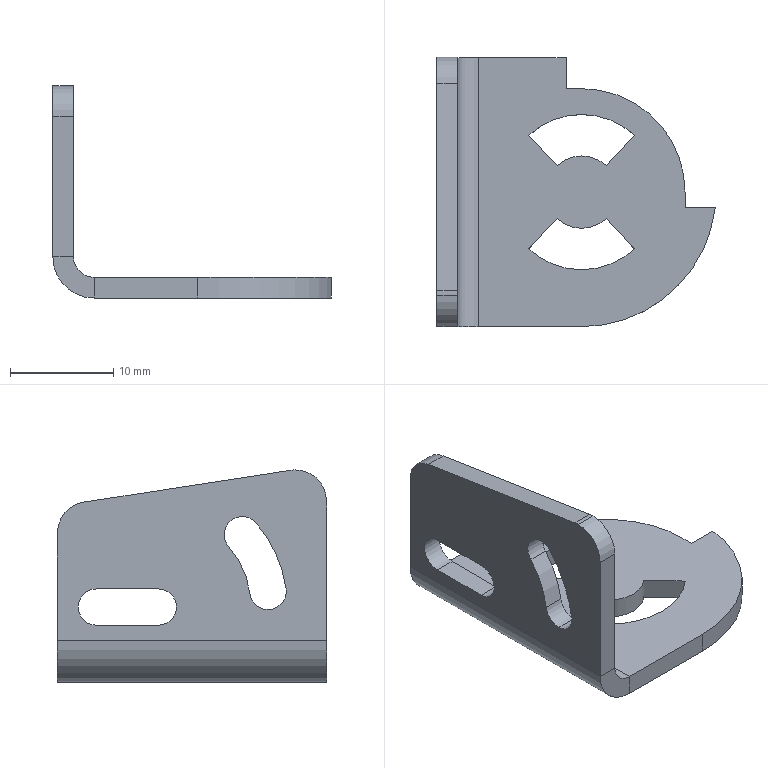Part | SolidWorks | features ICE 4, EdgeFlange 1, Fillet 1, FlatPattern 1, SMBaseFlange 1, SheetMetal 1 | 1 solid | 39 faces | box 26.913 x 26 x 20.503 mm | volume 1687 mm3 | plane 21 | cylinder 18 | commonest cylinder face diameters 3.5 x5 6 x3 7 x2 15 x2 4 x1 8 x1
STEP:
#1=CARTESIAN_POINT('',(-5.,-10.,18.503));
#2=VERTEX_POINT('',#1);
#3=CARTESIAN_POINT('',(-5.,-13.,15.503));
#4=VERTEX_POINT('',#3);
#5=CARTESIAN_POINT('',(-5.,-10.,15.503));
#6=DIRECTION('',(1.,0.,0.));
#7=DIRECTION('',(0.,0.,1.));
#8=AXIS2_PLACEMENT_3D('',#5,#6,#7);
#9=CIRCLE('',#8,3.);
#10=EDGE_CURVE('',#2,#4,#9,.T.);
#11=ORIENTED_EDGE('',*,*,#10,.F.);
#12=CARTESIAN_POINT('',(-7.,-10.,18.503));
#13=VERTEX_POINT('',#12);
#14=CARTESIAN_POINT('',(-7.,-10.,18.503));
#15=DIRECTION('',(-1.,0.,0.));
#16=VECTOR('',#15,1000.);
#17=LINE('',#14,#16);
#18=EDGE_CURVE('',#2,#13,#17,.T.);
#19=ORIENTED_EDGE('',*,*,#18,.T.);
#20=CARTESIAN_POINT('',(-7.,-13.,15.503));
#21=VERTEX_POINT('',#20);
#22=CARTESIAN_POINT('',(-7.,-10.,15.503));
#23=DIRECTION('',(-1.,0.,0.));
#24=DIRECTION('',(0.,0.,1.));
#25=AXIS2_PLACEMENT_3D('',#22,#23,#24);
#26=CIRCLE('',#25,3.);
#27=EDGE_CURVE('',#21,#13,#26,.T.);
#28=ORIENTED_EDGE('',*,*,#27,.F.);
#29=CARTESIAN_POINT('',(-7.,-13.,15.503));
#30=DIRECTION('',(-1.,0.,0.));
#31=VECTOR('',#30,1000.);
#32=LINE('',#29,#31);
#33=EDGE_CURVE('',#4,#21,#32,.T.);
#34=ORIENTED_EDGE('',*,*,#33,.F.);
#35=EDGE_LOOP('',(#11,#19,#28,#34));
#36=FACE_OUTER_BOUND('',#35,.T.);
#37=CARTESIAN_POINT('',(-7.,-10.,15.503));
#38=DIRECTION('',(-1.,0.,0.));
#39=DIRECTION('',(0.,0.,1.));
#40=AXIS2_PLACEMENT_3D('',#37,#38,#39);
#41=CYLINDRICAL_SURFACE('',#40,3.);
#42=ADVANCED_FACE('',(#36),#41,.T.);
#43=CARTESIAN_POINT('',(-7.,-7.354,5.));
#44=VERTEX_POINT('',#43);
#45=CARTESIAN_POINT('',(-7.,-5.621,6.505));
#46=VERTEX_POINT('',#45);
#47=CARTESIAN_POINT('',(-7.,-7.354,6.75));
#48=DIRECTION('',(1.,0.,0.));
#49=DIRECTION('',(0.,0.,-1.));
#50=AXIS2_PLACEMENT_3D('',#47,#48,#49);
#51=CIRCLE('',#50,1.75);
#52=EDGE_CURVE('',#44,#46,#51,.T.);
#53=ORIENTED_EDGE('',*,*,#52,.F.);
#54=CARTESIAN_POINT('',(-5.,-7.354,5.));
#55=VERTEX_POINT('',#54);
#56=CARTESIAN_POINT('',(-7.,-7.354,5.));
#57=DIRECTION('',(1.,0.,0.));
#58=VECTOR('',#57,1000.);
#59=LINE('',#56,#58);
#60=EDGE_CURVE('',#44,#55,#59,.T.);
#61=ORIENTED_EDGE('',*,*,#60,.T.);
#62=CARTESIAN_POINT('',(-5.,-5.621,6.505));
#63=VERTEX_POINT('',#62);
#64=CARTESIAN_POINT('',(-5.,-7.354,6.75));
#65=DIRECTION('',(1.,0.,0.));
#66=DIRECTION('',(0.,0.,-1.));
#67=AXIS2_PLACEMENT_3D('',#64,#65,#66);
#68=CIRCLE('',#67,1.75);
#69=EDGE_CURVE('',#55,#63,#68,.T.);
#70=ORIENTED_EDGE('',*,*,#69,.T.);
#71=CARTESIAN_POINT('',(-7.,-5.621,6.505));
#72=DIRECTION('',(1.,0.,0.));
#73=VECTOR('',#72,1000.);
#74=LINE('',#71,#73);
#75=EDGE_CURVE('',#46,#63,#74,.T.);
#76=ORIENTED_EDGE('',*,*,#75,.F.);
#77=EDGE_LOOP('',(#53,#61,#70,#76));
#78=FACE_OUTER_BOUND('',#77,.T.);
#79=CARTESIAN_POINT('',(-7.,-7.354,6.75));
#80=DIRECTION('',(1.,0.,0.));
#81=DIRECTION('',(0.,0.,-1.));
#82=AXIS2_PLACEMENT_3D('',#79,#80,#81);
#83=CYLINDRICAL_SURFACE('',#82,1.75);
#84=ADVANCED_FACE('',(#78),#83,.F.);
#85=CARTESIAN_POINT('',(-3.,-13.,0.));
#86=VERTEX_POINT('',#85);
#87=CARTESIAN_POINT('',(7.,-13.,0.));
#88=VERTEX_POINT('',#87);
#89=CARTESIAN_POINT('',(-7.,-13.,0.));
#90=DIRECTION('',(1.,0.,0.));
#91=VECTOR('',#90,1000.);
#92=LINE('',#89,#91);
#93=EDGE_CURVE('',#86,#88,#92,.T.);
#94=ORIENTED_EDGE('',*,*,#93,.F.);
#95=CARTESIAN_POINT('',(-3.,-13.,-2.));
#96=VERTEX_POINT('',#95);
#97=CARTESIAN_POINT('',(-3.,-13.,0.));
#98=DIRECTION('',(0.,0.,-1.));
#99=VECTOR('',#98,1000.);
#100=LINE('',#97,#99);
#101=EDGE_CURVE('',#86,#96,#100,.T.);
#102=ORIENTED_EDGE('',*,*,#101,.T.);
#103=CARTESIAN_POINT('',(7.,-13.,-2.));
#104=VERTEX_POINT('',#103);
#105=CARTESIAN_POINT('',(-7.,-13.,-2.));
#106=DIRECTION('',(1.,0.,0.));
#107=VECTOR('',#106,1000.);
#108=LINE('',#105,#107);
#109=EDGE_CURVE('',#96,#104,#108,.T.);
#110=ORIENTED_EDGE('',*,*,#109,.T.);
#111=CARTESIAN_POINT('',(7.,-13.,-2.));
#112=DIRECTION('',(0.,0.,1.));
#113=VECTOR('',#112,1000.);
#114=LINE('',#111,#113);
#115=EDGE_CURVE('',#104,#88,#114,.T.);
#116=ORIENTED_EDGE('',*,*,#115,.T.);
#117=EDGE_LOOP('',(#94,#102,#110,#116));
#118=FACE_OUTER_BOUND('',#117,.T.);
#119=CARTESIAN_POINT('',(-7.,-13.,-2.));
#120=DIRECTION('',(0.,-1.,0.));
#121=DIRECTION('',(0.,0.,-1.));
#122=AXIS2_PLACEMENT_3D('',#119,#120,#121);
#123=PLANE('',#122);
#124=ADVANCED_FACE('',(#118),#123,.T.);
#125=CARTESIAN_POINT('',(1.901,-5.5,-2.));
#126=VERTEX_POINT('',#125);
#127=CARTESIAN_POINT('',(12.099,-5.5,-2.));
#128=VERTEX_POINT('',#127);
#129=CARTESIAN_POINT('',(7.,0.,-2.));
#130=DIRECTION('',(0.,0.,1.));
#131=DIRECTION('',(-1.,0.,0.));
#132=AXIS2_PLACEMENT_3D('',#129,#130,#131);
#133=CIRCLE('',#132,7.5);
#134=EDGE_CURVE('',#126,#128,#133,.T.);
#135=ORIENTED_EDGE('',*,*,#134,.T.);
#136=CARTESIAN_POINT('',(9.38,-2.567,-2.));
#137=VERTEX_POINT('',#136);
#138=CARTESIAN_POINT('',(12.099,-5.5,-2.));
#139=DIRECTION('',(-0.6799,0.7333,0.));
#140=VECTOR('',#139,1000.);
#141=LINE('',#138,#140);
#142=EDGE_CURVE('',#128,#137,#141,.T.);
#143=ORIENTED_EDGE('',*,*,#142,.T.);
#144=CARTESIAN_POINT('',(4.62,-2.567,-2.));
#145=VERTEX_POINT('',#144);
#146=CARTESIAN_POINT('',(7.,0.,-2.));
#147=DIRECTION('',(0.,0.,-1.));
#148=DIRECTION('',(-1.,0.,0.));
#149=AXIS2_PLACEMENT_3D('',#146,#147,#148);
#150=CIRCLE('',#149,3.5);
#151=EDGE_CURVE('',#137,#145,#150,.T.);
#152=ORIENTED_EDGE('',*,*,#151,.T.);
#153=CARTESIAN_POINT('',(4.62,-2.567,-2.));
#154=DIRECTION('',(-0.6799,-0.7333,0.));
#155=VECTOR('',#154,1000.);
#156=LINE('',#153,#155);
#157=EDGE_CURVE('',#145,#126,#156,.T.);
#158=ORIENTED_EDGE('',*,*,#157,.T.);
#159=EDGE_LOOP('',(#135,#143,#152,#158));
#160=FACE_BOUND('',#159,.T.);
#161=CARTESIAN_POINT('',(4.62,2.567,-2.));
#162=VERTEX_POINT('',#161);
#163=CARTESIAN_POINT('',(9.38,2.567,-2.));
#164=VERTEX_POINT('',#163);
#165=CARTESIAN_POINT('',(7.,0.,-2.));
#166=DIRECTION('',(0.,0.,-1.));
#167=DIRECTION('',(1.,0.,0.));
#168=AXIS2_PLACEMENT_3D('',#165,#166,#167);
#169=CIRCLE('',#168,3.5);
#170=EDGE_CURVE('',#162,#164,#169,.T.);
#171=ORIENTED_EDGE('',*,*,#170,.T.);
#172=CARTESIAN_POINT('',(12.099,5.5,-2.));
#173=VERTEX_POINT('',#172);
#174=CARTESIAN_POINT('',(12.099,5.5,-2.));
#175=DIRECTION('',(0.6799,0.7333,0.));
#176=VECTOR('',#175,1000.);
#177=LINE('',#174,#176);
#178=EDGE_CURVE('',#164,#173,#177,.T.);
#179=ORIENTED_EDGE('',*,*,#178,.T.);
#180=CARTESIAN_POINT('',(1.901,5.5,-2.));
#181=VERTEX_POINT('',#180);
#182=CARTESIAN_POINT('',(7.,0.,-2.));
#183=DIRECTION('',(0.,0.,1.));
#184=DIRECTION('',(1.,0.,0.));
#185=AXIS2_PLACEMENT_3D('',#182,#183,#184);
#186=CIRCLE('',#185,7.5);
#187=EDGE_CURVE('',#173,#181,#186,.T.);
#188=ORIENTED_EDGE('',*,*,#187,.T.);
#189=CARTESIAN_POINT('',(4.62,2.567,-2.));
#190=DIRECTION('',(0.6799,-0.7333,0.));
#191=VECTOR('',#190,1000.);
#192=LINE('',#189,#191);
#193=EDGE_CURVE('',#181,#162,#192,.T.);
#194=ORIENTED_EDGE('',*,*,#193,.T.);
#195=EDGE_LOOP('',(#171,#179,#188,#194));
#196=FACE_BOUND('',#195,.T.);
#197=CARTESIAN_POINT('',(17.,-1.5,-2.));
#198=VERTEX_POINT('',#197);
#199=CARTESIAN_POINT('',(19.913,-1.5,-2.));
#200=VERTEX_POINT('',#199);
#201=CARTESIAN_POINT('',(17.,-1.5,-2.));
#202=DIRECTION('',(1.,0.,0.));
#203=VECTOR('',#202,1000.);
#204=LINE('',#201,#203);
#205=EDGE_CURVE('',#198,#200,#204,.T.);
#206=ORIENTED_EDGE('',*,*,#205,.T.);
#207=CARTESIAN_POINT('',(7.,0.,-2.));
#208=DIRECTION('',(0.,0.,1.));
#209=DIRECTION('',(-1.,0.,0.));
#210=AXIS2_PLACEMENT_3D('',#207,#208,#209);
#211=CIRCLE('',#210,13.);
#212=EDGE_CURVE('',#104,#200,#211,.T.);
#213=ORIENTED_EDGE('',*,*,#212,.F.);
#214=ORIENTED_EDGE('',*,*,#109,.F.);
#215=CARTESIAN_POINT('',(-3.,13.,-2.));
#216=VERTEX_POINT('',#215);
#217=CARTESIAN_POINT('',(-3.,-13.,-2.));
#218=DIRECTION('',(0.,1.,0.));
#219=VECTOR('',#218,1000.);
#220=LINE('',#217,#219);
#221=EDGE_CURVE('',#96,#216,#220,.T.);
#222=ORIENTED_EDGE('',*,*,#221,.T.);
#223=CARTESIAN_POINT('',(5.5,13.,-2.));
#224=VERTEX_POINT('',#223);
#225=CARTESIAN_POINT('',(-7.,13.,-2.));
#226=DIRECTION('',(-1.,0.,0.));
#227=VECTOR('',#226,1000.);
#228=LINE('',#225,#227);
#229=EDGE_CURVE('',#224,#216,#228,.T.);
#230=ORIENTED_EDGE('',*,*,#229,.F.);
#231=CARTESIAN_POINT('',(5.5,10.,-2.));
#232=VERTEX_POINT('',#231);
#233=CARTESIAN_POINT('',(5.5,13.,-2.));
#234=DIRECTION('',(0.,-1.,0.));
#235=VECTOR('',#234,1000.);
#236=LINE('',#233,#235);
#237=EDGE_CURVE('',#224,#232,#236,.T.);
#238=ORIENTED_EDGE('',*,*,#237,.T.);
#239=CARTESIAN_POINT('',(7.,10.,-2.));
#240=VERTEX_POINT('',#239);
#241=CARTESIAN_POINT('',(5.5,10.,-2.));
#242=DIRECTION('',(1.,0.,0.));
#243=VECTOR('',#242,1000.);
#244=LINE('',#241,#243);
#245=EDGE_CURVE('',#232,#240,#244,.T.);
#246=ORIENTED_EDGE('',*,*,#245,.T.);
#247=CARTESIAN_POINT('',(17.,0.,-2.));
#248=VERTEX_POINT('',#247);
#249=CARTESIAN_POINT('',(7.,0.,-2.));
#250=DIRECTION('',(0.,0.,-1.));
#251=DIRECTION('',(1.,0.,0.));
#252=AXIS2_PLACEMENT_3D('',#249,#250,#251);
#253=CIRCLE('',#252,10.);
#254=EDGE_CURVE('',#240,#248,#253,.T.);
#255=ORIENTED_EDGE('',*,*,#254,.T.);
#256=CARTESIAN_POINT('',(17.,0.,-2.));
#257=DIRECTION('',(0.,-1.,0.));
#258=VECTOR('',#257,1000.);
#259=LINE('',#256,#258);
#260=EDGE_CURVE('',#248,#198,#259,.T.);
#261=ORIENTED_EDGE('',*,*,#260,.T.);
#262=EDGE_LOOP('',(#206,#213,#214,#222,#230,#238,#246,#255,#261));
#263=FACE_OUTER_BOUND('',#262,.T.);
#264=CARTESIAN_POINT('',(7.,0.,-2.));
#265=DIRECTION('',(0.,0.,-1.));
#266=DIRECTION('',(-1.,0.,0.));
#267=AXIS2_PLACEMENT_3D('',#264,#265,#266);
#268=PLANE('',#267);
#269=ADVANCED_FACE('',(#160,#196,#263),#268,.T.);
#270=CARTESIAN_POINT('',(12.099,-5.5,0.));
#271=VERTEX_POINT('',#270);
#272=CARTESIAN_POINT('',(9.38,-2.567,0.));
#273=VERTEX_POINT('',#272);
#274=CARTESIAN_POINT('',(12.099,-5.5,0.));
#275=DIRECTION('',(-0.6799,0.7333,0.));
#276=VECTOR('',#275,1000.);
#277=LINE('',#274,#276);
#278=EDGE_CURVE('',#271,#273,#277,.T.);
#279=ORIENTED_EDGE('',*,*,#278,.F.);
#280=CARTESIAN_POINT('',(1.901,-5.5,0.));
#281=VERTEX_POINT('',#280);
#282=CARTESIAN_POINT('',(7.,0.,0.));
#283=DIRECTION('',(0.,0.,1.));
#284=DIRECTION('',(-1.,0.,0.));
#285=AXIS2_PLACEMENT_3D('',#282,#283,#284);
#286=CIRCLE('',#285,7.5);
#287=EDGE_CURVE('',#281,#271,#286,.T.);
#288=ORIENTED_EDGE('',*,*,#287,.F.);
#289=CARTESIAN_POINT('',(4.62,-2.567,0.));
#290=VERTEX_POINT('',#289);
#291=CARTESIAN_POINT('',(4.62,-2.567,0.));
#292=DIRECTION('',(-0.6799,-0.7333,0.));
#293=VECTOR('',#292,1000.);
#294=LINE('',#291,#293);
#295=EDGE_CURVE('',#290,#281,#294,.T.);
#296=ORIENTED_EDGE('',*,*,#295,.F.);
#297=CARTESIAN_POINT('',(7.,0.,0.));
#298=DIRECTION('',(0.,0.,-1.));
#299=DIRECTION('',(-1.,0.,0.));
#300=AXIS2_PLACEMENT_3D('',#297,#298,#299);
#301=CIRCLE('',#300,3.5);
#302=EDGE_CURVE('',#273,#290,#301,.T.);
#303=ORIENTED_EDGE('',*,*,#302,.F.);
#304=EDGE_LOOP('',(#279,#288,#296,#303));
#305=FACE_BOUND('',#304,.T.);
#306=CARTESIAN_POINT('',(9.38,2.567,0.));
#307=VERTEX_POINT('',#306);
#308=CARTESIAN_POINT('',(12.099,5.5,0.));
#309=VERTEX_POINT('',#308);
#310=CARTESIAN_POINT('',(12.099,5.5,0.));
#311=DIRECTION('',(0.6799,0.7333,0.));
#312=VECTOR('',#311,1000.);
#313=LINE('',#310,#312);
#314=EDGE_CURVE('',#307,#309,#313,.T.);
#315=ORIENTED_EDGE('',*,*,#314,.F.);
#316=CARTESIAN_POINT('',(4.62,2.567,0.));
#317=VERTEX_POINT('',#316);
#318=CARTESIAN_POINT('',(7.,0.,0.));
#319=DIRECTION('',(0.,0.,-1.));
#320=DIRECTION('',(1.,0.,0.));
#321=AXIS2_PLACEMENT_3D('',#318,#319,#320);
#322=CIRCLE('',#321,3.5);
#323=EDGE_CURVE('',#317,#307,#322,.T.);
#324=ORIENTED_EDGE('',*,*,#323,.F.);
#325=CARTESIAN_POINT('',(1.901,5.5,0.));
#326=VERTEX_POINT('',#325);
#327=CARTESIAN_POINT('',(4.62,2.567,0.));
#328=DIRECTION('',(0.6799,-0.7333,0.));
#329=VECTOR('',#328,1000.);
#330=LINE('',#327,#329);
#331=EDGE_CURVE('',#326,#317,#330,.T.);
#332=ORIENTED_EDGE('',*,*,#331,.F.);
#333=CARTESIAN_POINT('',(7.,0.,0.));
#334=DIRECTION('',(0.,0.,1.));
#335=DIRECTION('',(1.,0.,0.));
#336=AXIS2_PLACEMENT_3D('',#333,#334,#335);
#337=CIRCLE('',#336,7.5);
#338=EDGE_CURVE('',#309,#326,#337,.T.);
#339=ORIENTED_EDGE('',*,*,#338,.F.);
#340=EDGE_LOOP('',(#315,#324,#332,#339));
#341=FACE_BOUND('',#340,.T.);
#342=CARTESIAN_POINT('',(19.913,-1.5,0.));
#343=VERTEX_POINT('',#342);
#344=CARTESIAN_POINT('',(7.,0.,0.));
#345=DIRECTION('',(0.,0.,1.));
#346=DIRECTION('',(-1.,0.,0.));
#347=AXIS2_PLACEMENT_3D('',#344,#345,#346);
#348=CIRCLE('',#347,13.);
#349=EDGE_CURVE('',#88,#343,#348,.T.);
#350=ORIENTED_EDGE('',*,*,#349,.T.);
#351=CARTESIAN_POINT('',(17.,-1.5,0.));
#352=VERTEX_POINT('',#351);
#353=CARTESIAN_POINT('',(17.,-1.5,0.));
#354=DIRECTION('',(1.,0.,0.));
#355=VECTOR('',#354,1000.);
#356=LINE('',#353,#355);
#357=EDGE_CURVE('',#352,#343,#356,.T.);
#358=ORIENTED_EDGE('',*,*,#357,.F.);
#359=CARTESIAN_POINT('',(17.,0.,0.));
#360=VERTEX_POINT('',#359);
#361=CARTESIAN_POINT('',(17.,0.,0.));
#362=DIRECTION('',(0.,-1.,0.));
#363=VECTOR('',#362,1000.);
#364=LINE('',#361,#363);
#365=EDGE_CURVE('',#360,#352,#364,.T.);
#366=ORIENTED_EDGE('',*,*,#365,.F.);
#367=CARTESIAN_POINT('',(7.,10.,0.));
#368=VERTEX_POINT('',#367);
#369=CARTESIAN_POINT('',(7.,0.,0.));
#370=DIRECTION('',(0.,0.,-1.));
#371=DIRECTION('',(1.,0.,0.));
#372=AXIS2_PLACEMENT_3D('',#369,#370,#371);
#373=CIRCLE('',#372,10.);
#374=EDGE_CURVE('',#368,#360,#373,.T.);
#375=ORIENTED_EDGE('',*,*,#374,.F.);
#376=CARTESIAN_POINT('',(5.5,10.,0.));
#377=VERTEX_POINT('',#376);
#378=CARTESIAN_POINT('',(5.5,10.,0.));
#379=DIRECTION('',(1.,0.,0.));
#380=VECTOR('',#379,1000.);
#381=LINE('',#378,#380);
#382=EDGE_CURVE('',#377,#368,#381,.T.);
#383=ORIENTED_EDGE('',*,*,#382,.F.);
#384=CARTESIAN_POINT('',(5.5,13.,0.));
#385=VERTEX_POINT('',#384);
#386=CARTESIAN_POINT('',(5.5,13.,0.));
#387=DIRECTION('',(0.,-1.,0.));
#388=VECTOR('',#387,1000.);
#389=LINE('',#386,#388);
#390=EDGE_CURVE('',#385,#377,#389,.T.);
#391=ORIENTED_EDGE('',*,*,#390,.F.);
#392=CARTESIAN_POINT('',(-3.,13.,0.));
#393=VERTEX_POINT('',#392);
#394=CARTESIAN_POINT('',(-7.,13.,0.));
#395=DIRECTION('',(-1.,0.,0.));
#396=VECTOR('',#395,1000.);
#397=LINE('',#394,#396);
#398=EDGE_CURVE('',#385,#393,#397,.T.);
#399=ORIENTED_EDGE('',*,*,#398,.T.);
#400=CARTESIAN_POINT('',(-3.,-13.,0.));
#401=DIRECTION('',(0.,1.,0.));
#402=VECTOR('',#401,1000.);
#403=LINE('',#400,#402);
#404=EDGE_CURVE('',#86,#393,#403,.T.);
#405=ORIENTED_EDGE('',*,*,#404,.F.);
#406=ORIENTED_EDGE('',*,*,#93,.T.);
#407=EDGE_LOOP('',(#350,#358,#366,#375,#383,#391,#399,#405,#406));
#408=FACE_OUTER_BOUND('',#407,.T.);
#409=CARTESIAN_POINT('',(7.,0.,0.));
#410=DIRECTION('',(0.,0.,-1.));
#411=DIRECTION('',(-1.,0.,0.));
#412=AXIS2_PLACEMENT_3D('',#409,#410,#411);
#413=PLANE('',#412);
#414=ADVANCED_FACE('',(#305,#341,#408),#413,.F.);
#415=CARTESIAN_POINT('',(19.913,-1.5,-2.));
#416=DIRECTION('',(0.,0.,1.));
#417=VECTOR('',#416,1000.);
#418=LINE('',#415,#417);
#419=EDGE_CURVE('',#200,#343,#418,.T.);
#420=ORIENTED_EDGE('',*,*,#419,.T.);
#421=ORIENTED_EDGE('',*,*,#349,.F.);
#422=ORIENTED_EDGE('',*,*,#115,.F.);
#423=ORIENTED_EDGE('',*,*,#212,.T.);
#424=EDGE_LOOP('',(#420,#421,#422,#423));
#425=FACE_OUTER_BOUND('',#424,.T.);
#426=CARTESIAN_POINT('',(7.,0.,-2.));
#427=DIRECTION('',(0.,0.,1.));
#428=DIRECTION('',(1.,0.,0.));
#429=AXIS2_PLACEMENT_3D('',#426,#427,#428);
#430=CYLINDRICAL_SURFACE('',#429,13.);
#431=ADVANCED_FACE('',(#425),#430,.T.);
#432=CARTESIAN_POINT('',(5.5,13.,-2.));
#433=DIRECTION('',(0.,0.,1.));
#434=VECTOR('',#433,1000.);
#435=LINE('',#432,#434);
#436=EDGE_CURVE('',#224,#385,#435,.T.);
#437=ORIENTED_EDGE('',*,*,#436,.F.);
#438=ORIENTED_EDGE('',*,*,#229,.T.);
#439=CARTESIAN_POINT('',(-3.,13.,0.));
#440=DIRECTION('',(0.,0.,-1.));
#441=VECTOR('',#440,1000.);
#442=LINE('',#439,#441);
#443=EDGE_CURVE('',#393,#216,#442,.T.);
#444=ORIENTED_EDGE('',*,*,#443,.F.);
#445=ORIENTED_EDGE('',*,*,#398,.F.);
#446=EDGE_LOOP('',(#437,#438,#444,#445));
#447=FACE_OUTER_BOUND('',#446,.T.);
#448=CARTESIAN_POINT('',(-7.,13.,-2.));
#449=DIRECTION('',(0.,1.,0.));
#450=DIRECTION('',(0.,0.,1.));
#451=AXIS2_PLACEMENT_3D('',#448,#449,#450);
#452=PLANE('',#451);
#453=ADVANCED_FACE('',(#447),#452,.T.);
#454=CARTESIAN_POINT('',(-5.,13.,2.));
#455=VERTEX_POINT('',#454);
#456=CARTESIAN_POINT('',(-7.,13.,2.));
#457=VERTEX_POINT('',#456);
#458=CARTESIAN_POINT('',(-7.,13.,2.));
#459=DIRECTION('',(-1.,0.,0.));
#460=VECTOR('',#459,1000.);
#461=LINE('',#458,#460);
#462=EDGE_CURVE('',#455,#457,#461,.T.);
#463=ORIENTED_EDGE('',*,*,#462,.F.);
#464=CARTESIAN_POINT('',(-3.,13.,2.));
#465=DIRECTION('',(0.,1.,0.));
#466=DIRECTION('',(0.,0.,-1.));
#467=AXIS2_PLACEMENT_3D('',#464,#465,#466);
#468=CIRCLE('',#467,2.);
#469=EDGE_CURVE('',#393,#455,#468,.T.);
#470=ORIENTED_EDGE('',*,*,#469,.F.);
#471=ORIENTED_EDGE('',*,*,#443,.T.);
#472=CARTESIAN_POINT('',(-3.,13.,2.));
#473=DIRECTION('',(0.,1.,0.));
#474=DIRECTION('',(0.,0.,-1.));
#475=AXIS2_PLACEMENT_3D('',#472,#473,#474);
#476=CIRCLE('',#475,4.);
#477=EDGE_CURVE('',#216,#457,#476,.T.);
#478=ORIENTED_EDGE('',*,*,#477,.T.);
#479=EDGE_LOOP('',(#463,#470,#471,#478));
#480=FACE_OUTER_BOUND('',#479,.T.);
#481=CARTESIAN_POINT('',(-3.,13.,2.));
#482=DIRECTION('',(0.,1.,0.));
#483=DIRECTION('',(0.,0.,1.));
#484=AXIS2_PLACEMENT_3D('',#481,#482,#483);
#485=PLANE('',#484);
#486=ADVANCED_FACE('',(#480),#485,.T.);
#487=CARTESIAN_POINT('',(-5.,-13.,2.));
#488=VERTEX_POINT('',#487);
#489=CARTESIAN_POINT('',(-3.,-13.,2.));
#490=DIRECTION('',(0.,-1.,0.));
#491=DIRECTION('',(0.,0.,-1.));
#492=AXIS2_PLACEMENT_3D('',#489,#490,#491);
#493=CIRCLE('',#492,2.);
#494=EDGE_CURVE('',#488,#86,#493,.T.);
#495=ORIENTED_EDGE('',*,*,#494,.F.);
#496=CARTESIAN_POINT('',(-7.,-13.,2.));
#497=VERTEX_POINT('',#496);
#498=CARTESIAN_POINT('',(-5.,-13.,2.));
#499=DIRECTION('',(-1.,0.,0.));
#500=VECTOR('',#499,1000.);
#501=LINE('',#498,#500);
#502=EDGE_CURVE('',#488,#497,#501,.T.);
#503=ORIENTED_EDGE('',*,*,#502,.T.);
#504=CARTESIAN_POINT('',(-3.,-13.,2.));
#505=DIRECTION('',(0.,-1.,0.));
#506=DIRECTION('',(0.,0.,-1.));
#507=AXIS2_PLACEMENT_3D('',#504,#505,#506);
#508=CIRCLE('',#507,4.);
#509=EDGE_CURVE('',#497,#96,#508,.T.);
#510=ORIENTED_EDGE('',*,*,#509,.T.);
#511=ORIENTED_EDGE('',*,*,#101,.F.);
#512=EDGE_LOOP('',(#495,#503,#510,#511));
#513=FACE_OUTER_BOUND('',#512,.T.);
#514=CARTESIAN_POINT('',(-3.,-13.,2.));
#515=DIRECTION('',(0.,1.,0.));
#516=DIRECTION('',(0.,0.,1.));
#517=AXIS2_PLACEMENT_3D('',#514,#515,#516);
#518=PLANE('',#517);
#519=ADVANCED_FACE('',(#513),#518,.F.);
#520=ORIENTED_EDGE('',*,*,#221,.F.);
#521=ORIENTED_EDGE('',*,*,#509,.F.);
#522=CARTESIAN_POINT('',(-7.,0.,2.));
#523=DIRECTION('',(0.,-1.,0.));
#524=VECTOR('',#523,1000.);
#525=LINE('',#522,#524);
#526=EDGE_CURVE('',#457,#497,#525,.T.);
#527=ORIENTED_EDGE('',*,*,#526,.F.);
#528=ORIENTED_EDGE('',*,*,#477,.F.);
#529=EDGE_LOOP('',(#520,#521,#527,#528));
#530=FACE_OUTER_BOUND('',#529,.T.);
#531=CARTESIAN_POINT('',(-3.,-13.,2.));
#532=DIRECTION('',(0.,-1.,0.));
#533=DIRECTION('',(-1.,0.,0.));
#534=AXIS2_PLACEMENT_3D('',#531,#532,#533);
#535=CYLINDRICAL_SURFACE('',#534,4.);
#536=ADVANCED_FACE('',(#530),#535,.T.);
#537=ORIENTED_EDGE('',*,*,#404,.T.);
#538=ORIENTED_EDGE('',*,*,#469,.T.);
#539=CARTESIAN_POINT('',(-5.,13.,2.));
#540=DIRECTION('',(0.,-1.,0.));
#541=VECTOR('',#540,1000.);
#542=LINE('',#539,#541);
#543=EDGE_CURVE('',#455,#488,#542,.T.);
#544=ORIENTED_EDGE('',*,*,#543,.T.);
#545=ORIENTED_EDGE('',*,*,#494,.T.);
#546=EDGE_LOOP('',(#537,#538,#544,#545));
#547=FACE_OUTER_BOUND('',#546,.T.);
#548=CARTESIAN_POINT('',(-3.,-13.,2.));
#549=DIRECTION('',(0.,-1.,0.));
#550=DIRECTION('',(-1.,0.,0.));
#551=AXIS2_PLACEMENT_3D('',#548,#549,#550);
#552=CYLINDRICAL_SURFACE('',#551,2.);
#553=ADVANCED_FACE('',(#547),#552,.F.);
#554=CARTESIAN_POINT('',(-5.,-13.,0.));
#555=DIRECTION('',(0.,0.,-1.));
#556=VECTOR('',#555,1000.);
#557=LINE('',#554,#556);
#558=EDGE_CURVE('',#4,#488,#557,.T.);
#559=ORIENTED_EDGE('',*,*,#558,.F.);
#560=ORIENTED_EDGE('',*,*,#33,.T.);
#561=CARTESIAN_POINT('',(-7.,-13.,0.));
#562=DIRECTION('',(0.,0.,-1.));
#563=VECTOR('',#562,1000.);
#564=LINE('',#561,#563);
#565=EDGE_CURVE('',#21,#497,#564,.T.);
#566=ORIENTED_EDGE('',*,*,#565,.T.);
#567=ORIENTED_EDGE('',*,*,#502,.F.);
#568=EDGE_LOOP('',(#559,#560,#566,#567));
#569=FACE_OUTER_BOUND('',#568,.T.);
#570=CARTESIAN_POINT('',(-7.,-13.,0.));
#571=DIRECTION('',(0.,-1.,0.));
#572=DIRECTION('',(0.,0.,-1.));
#573=AXIS2_PLACEMENT_3D('',#570,#571,#572);
#574=PLANE('',#573);
#575=ADVANCED_FACE('',(#569),#574,.T.);
#576=CARTESIAN_POINT('',(-7.,13.,12.426));
#577=VERTEX_POINT('',#576);
#578=CARTESIAN_POINT('',(-7.,13.,19.));
#579=DIRECTION('',(0.,0.,1.));
#580=VECTOR('',#579,1000.);
#581=LINE('',#578,#580);
#582=EDGE_CURVE('',#457,#577,#581,.T.);
#583=ORIENTED_EDGE('',*,*,#582,.T.);
#584=CARTESIAN_POINT('',(-5.,13.,12.426));
#585=VERTEX_POINT('',#584);
#586=CARTESIAN_POINT('',(-5.,13.,12.426));
#587=DIRECTION('',(1.,0.,0.));
#588=VECTOR('',#587,1000.);
#589=LINE('',#586,#588);
#590=EDGE_CURVE('',#577,#585,#589,.T.);
#591=ORIENTED_EDGE('',*,*,#590,.T.);
#592=CARTESIAN_POINT('',(-5.,13.,0.));
#593=DIRECTION('',(0.,0.,1.));
#594=VECTOR('',#593,1000.);
#595=LINE('',#592,#594);
#596=EDGE_CURVE('',#455,#585,#595,.T.);
#597=ORIENTED_EDGE('',*,*,#596,.F.);
#598=ORIENTED_EDGE('',*,*,#462,.T.);
#599=EDGE_LOOP('',(#583,#591,#597,#598));
#600=FACE_OUTER_BOUND('',#599,.T.);
#601=CARTESIAN_POINT('',(-7.,13.,19.));
#602=DIRECTION('',(0.,1.,0.));
#603=DIRECTION('',(0.,0.,1.));
#604=AXIS2_PLACEMENT_3D('',#601,#602,#603);
#605=PLANE('',#604);
#606=ADVANCED_FACE('',(#600),#605,.T.);
#607=CARTESIAN_POINT('',(-7.,-9.544,18.468));
#608=VERTEX_POINT('',#607);
#609=CARTESIAN_POINT('',(-7.,10.456,15.391));
#610=VERTEX_POINT('',#609);
#611=CARTESIAN_POINT('',(-7.,-13.,19.));
#612=DIRECTION('',(0.,0.9884,-0.1521));
#613=VECTOR('',#612,1000.);
#614=LINE('',#611,#613);
#615=EDGE_CURVE('',#608,#610,#614,.T.);
#616=ORIENTED_EDGE('',*,*,#615,.T.);
#617=CARTESIAN_POINT('',(-7.,10.,12.426));
#618=DIRECTION('',(-1.,0.,0.));
#619=DIRECTION('',(0.,0.,1.));
#620=AXIS2_PLACEMENT_3D('',#617,#618,#619);
#621=CIRCLE('',#620,3.);
#622=EDGE_CURVE('',#610,#577,#621,.T.);
#623=ORIENTED_EDGE('',*,*,#622,.T.);
#624=ORIENTED_EDGE('',*,*,#582,.F.);
#625=ORIENTED_EDGE('',*,*,#526,.T.);
#626=ORIENTED_EDGE('',*,*,#565,.F.);
#627=ORIENTED_EDGE('',*,*,#27,.T.);
#628=CARTESIAN_POINT('',(-7.,-10.,15.503));
#629=DIRECTION('',(-1.,0.,0.));
#630=DIRECTION('',(0.,0.,1.));
#631=AXIS2_PLACEMENT_3D('',#628,#629,#630);
#632=CIRCLE('',#631,3.);
#633=EDGE_CURVE('',#13,#608,#632,.T.);
#634=ORIENTED_EDGE('',*,*,#633,.T.);
#635=EDGE_LOOP('',(#616,#623,#624,#625,#626,#627,#634));
#636=FACE_OUTER_BOUND('',#635,.T.);
#637=CARTESIAN_POINT('',(-7.,-3.53,11.106));
#638=VERTEX_POINT('',#637);
#639=CARTESIAN_POINT('',(-7.,-6.179,13.394));
#640=VERTEX_POINT('',#639);
#641=CARTESIAN_POINT('',(-7.,-4.855,12.25));
#642=DIRECTION('',(1.,0.,0.));
#643=DIRECTION('',(0.,0.,-1.));
#644=AXIS2_PLACEMENT_3D('',#641,#642,#643);
#645=CIRCLE('',#644,1.75);
#646=EDGE_CURVE('',#638,#640,#645,.T.);
#647=ORIENTED_EDGE('',*,*,#646,.T.);
#648=CARTESIAN_POINT('',(-7.,-9.086,6.995));
#649=VERTEX_POINT('',#648);
#650=CARTESIAN_POINT('',(-7.,3.25,5.25));
#651=DIRECTION('',(1.,0.,0.));
#652=DIRECTION('',(0.,0.,-1.));
#653=AXIS2_PLACEMENT_3D('',#650,#651,#652);
#654=CIRCLE('',#653,12.459);
#655=EDGE_CURVE('',#640,#649,#654,.T.);
#656=ORIENTED_EDGE('',*,*,#655,.T.);
#657=CARTESIAN_POINT('',(-7.,-7.354,6.75));
#658=DIRECTION('',(1.,0.,0.));
#659=DIRECTION('',(0.,0.,-1.));
#660=AXIS2_PLACEMENT_3D('',#657,#658,#659);
#661=CIRCLE('',#660,1.75);
#662=EDGE_CURVE('',#649,#44,#661,.T.);
#663=ORIENTED_EDGE('',*,*,#662,.T.);
#664=ORIENTED_EDGE('',*,*,#52,.T.);
#665=CARTESIAN_POINT('',(-7.,3.25,5.25));
#666=DIRECTION('',(-1.,0.,0.));
#667=DIRECTION('',(0.,0.,-1.));
#668=AXIS2_PLACEMENT_3D('',#665,#666,#667);
#669=CIRCLE('',#668,8.959);
#670=EDGE_CURVE('',#46,#638,#669,.T.);
#671=ORIENTED_EDGE('',*,*,#670,.T.);
#672=EDGE_LOOP('',(#647,#656,#663,#664,#671));
#673=FACE_BOUND('',#672,.T.);
#674=CARTESIAN_POINT('',(-7.,3.25,7.));
#675=VERTEX_POINT('',#674);
#676=CARTESIAN_POINT('',(-7.,3.25,3.5));
#677=VERTEX_POINT('',#676);
#678=CARTESIAN_POINT('',(-7.,3.25,5.25));
#679=DIRECTION('',(1.,0.,0.));
#680=DIRECTION('',(0.,0.,-1.));
#681=AXIS2_PLACEMENT_3D('',#678,#679,#680);
#682=CIRCLE('',#681,1.75);
#683=EDGE_CURVE('',#675,#677,#682,.T.);
#684=ORIENTED_EDGE('',*,*,#683,.T.);
#685=CARTESIAN_POINT('',(-7.,9.25,3.5));
#686=VERTEX_POINT('',#685);
#687=CARTESIAN_POINT('',(-7.,3.25,3.5));
#688=DIRECTION('',(0.,1.,0.));
#689=VECTOR('',#688,1000.);
#690=LINE('',#687,#689);
#691=EDGE_CURVE('',#677,#686,#690,.T.);
#692=ORIENTED_EDGE('',*,*,#691,.T.);
#693=CARTESIAN_POINT('',(-7.,9.25,7.));
#694=VERTEX_POINT('',#693);
#695=CARTESIAN_POINT('',(-7.,9.25,5.25));
#696=DIRECTION('',(1.,0.,0.));
#697=DIRECTION('',(0.,0.,-1.));
#698=AXIS2_PLACEMENT_3D('',#695,#696,#697);
#699=CIRCLE('',#698,1.75);
#700=EDGE_CURVE('',#686,#694,#699,.T.);
#701=ORIENTED_EDGE('',*,*,#700,.T.);
#702=CARTESIAN_POINT('',(-7.,3.25,7.));
#703=DIRECTION('',(0.,-1.,0.));
#704=VECTOR('',#703,1000.);
#705=LINE('',#702,#704);
#706=EDGE_CURVE('',#694,#675,#705,.T.);
#707=ORIENTED_EDGE('',*,*,#706,.T.);
#708=EDGE_LOOP('',(#684,#692,#701,#707));
#709=FACE_BOUND('',#708,.T.);
#710=CARTESIAN_POINT('',(-7.,0.,0.));
#711=DIRECTION('',(-1.,0.,0.));
#712=DIRECTION('',(0.,0.,1.));
#713=AXIS2_PLACEMENT_3D('',#710,#711,#712);
#714=PLANE('',#713);
#715=ADVANCED_FACE('',(#636,#673,#709),#714,.T.);
#716=CARTESIAN_POINT('',(-5.,-6.179,13.394));
#717=VERTEX_POINT('',#716);
#718=CARTESIAN_POINT('',(-5.,-9.086,6.995));
#719=VERTEX_POINT('',#718);
#720=CARTESIAN_POINT('',(-5.,3.25,5.25));
#721=DIRECTION('',(1.,0.,0.));
#722=DIRECTION('',(0.,0.,-1.));
#723=AXIS2_PLACEMENT_3D('',#720,#721,#722);
#724=CIRCLE('',#723,12.459);
#725=EDGE_CURVE('',#717,#719,#724,.T.);
#726=ORIENTED_EDGE('',*,*,#725,.F.);
#727=CARTESIAN_POINT('',(-5.,-3.53,11.106));
#728=VERTEX_POINT('',#727);
#729=CARTESIAN_POINT('',(-5.,-4.855,12.25));
#730=DIRECTION('',(1.,0.,0.));
#731=DIRECTION('',(0.,0.,-1.));
#732=AXIS2_PLACEMENT_3D('',#729,#730,#731);
#733=CIRCLE('',#732,1.75);
#734=EDGE_CURVE('',#728,#717,#733,.T.);
#735=ORIENTED_EDGE('',*,*,#734,.F.);
#736=CARTESIAN_POINT('',(-5.,3.25,5.25));
#737=DIRECTION('',(-1.,0.,0.));
#738=DIRECTION('',(0.,0.,-1.));
#739=AXIS2_PLACEMENT_3D('',#736,#737,#738);
#740=CIRCLE('',#739,8.959);
#741=EDGE_CURVE('',#63,#728,#740,.T.);
#742=ORIENTED_EDGE('',*,*,#741,.F.);
#743=ORIENTED_EDGE('',*,*,#69,.F.);
#744=CARTESIAN_POINT('',(-5.,-7.354,6.75));
#745=DIRECTION('',(1.,0.,0.));
#746=DIRECTION('',(0.,0.,-1.));
#747=AXIS2_PLACEMENT_3D('',#744,#745,#746);
#748=CIRCLE('',#747,1.75);
#749=EDGE_CURVE('',#719,#55,#748,.T.);
#750=ORIENTED_EDGE('',*,*,#749,.F.);
#751=EDGE_LOOP('',(#726,#735,#742,#743,#750));
#752=FACE_BOUND('',#751,.T.);
#753=CARTESIAN_POINT('',(-5.,3.25,3.5));
#754=VERTEX_POINT('',#753);
#755=CARTESIAN_POINT('',(-5.,9.25,3.5));
#756=VERTEX_POINT('',#755);
#757=CARTESIAN_POINT('',(-5.,3.25,3.5));
#758=DIRECTION('',(0.,1.,0.));
#759=VECTOR('',#758,1000.);
#760=LINE('',#757,#759);
#761=EDGE_CURVE('',#754,#756,#760,.T.);
#762=ORIENTED_EDGE('',*,*,#761,.F.);
#763=CARTESIAN_POINT('',(-5.,3.25,7.));
#764=VERTEX_POINT('',#763);
#765=CARTESIAN_POINT('',(-5.,3.25,5.25));
#766=DIRECTION('',(1.,0.,0.));
#767=DIRECTION('',(0.,0.,-1.));
#768=AXIS2_PLACEMENT_3D('',#765,#766,#767);
#769=CIRCLE('',#768,1.75);
#770=EDGE_CURVE('',#764,#754,#769,.T.);
#771=ORIENTED_EDGE('',*,*,#770,.F.);
#772=CARTESIAN_POINT('',(-5.,9.25,7.));
#773=VERTEX_POINT('',#772);
#774=CARTESIAN_POINT('',(-5.,3.25,7.));
#775=DIRECTION('',(0.,-1.,0.));
#776=VECTOR('',#775,1000.);
#777=LINE('',#774,#776);
#778=EDGE_CURVE('',#773,#764,#777,.T.);
#779=ORIENTED_EDGE('',*,*,#778,.F.);
#780=CARTESIAN_POINT('',(-5.,9.25,5.25));
#781=DIRECTION('',(1.,0.,0.));
#782=DIRECTION('',(0.,0.,-1.));
#783=AXIS2_PLACEMENT_3D('',#780,#781,#782);
#784=CIRCLE('',#783,1.75);
#785=EDGE_CURVE('',#756,#773,#784,.T.);
#786=ORIENTED_EDGE('',*,*,#785,.F.);
#787=EDGE_LOOP('',(#762,#771,#779,#786));
#788=FACE_BOUND('',#787,.T.);
#789=ORIENTED_EDGE('',*,*,#596,.T.);
#790=CARTESIAN_POINT('',(-5.,10.456,15.391));
#791=VERTEX_POINT('',#790);
#792=CARTESIAN_POINT('',(-5.,10.,12.426));
#793=DIRECTION('',(1.,0.,0.));
#794=DIRECTION('',(0.,0.,1.));
#795=AXIS2_PLACEMENT_3D('',#792,#793,#794);
#796=CIRCLE('',#795,3.);
#797=EDGE_CURVE('',#585,#791,#796,.T.);
#798=ORIENTED_EDGE('',*,*,#797,.T.);
#799=CARTESIAN_POINT('',(-5.,-9.544,18.468));
#800=VERTEX_POINT('',#799);
#801=CARTESIAN_POINT('',(-5.,-13.,19.));
#802=DIRECTION('',(0.,0.9884,-0.1521));
#803=VECTOR('',#802,1000.);
#804=LINE('',#801,#803);
#805=EDGE_CURVE('',#800,#791,#804,.T.);
#806=ORIENTED_EDGE('',*,*,#805,.F.);
#807=CARTESIAN_POINT('',(-5.,-10.,15.503));
#808=DIRECTION('',(1.,0.,0.));
#809=DIRECTION('',(0.,0.,1.));
#810=AXIS2_PLACEMENT_3D('',#807,#808,#809);
#811=CIRCLE('',#810,3.);
#812=EDGE_CURVE('',#800,#2,#811,.T.);
#813=ORIENTED_EDGE('',*,*,#812,.T.);
#814=ORIENTED_EDGE('',*,*,#10,.T.);
#815=ORIENTED_EDGE('',*,*,#558,.T.);
#816=ORIENTED_EDGE('',*,*,#543,.F.);
#817=EDGE_LOOP('',(#789,#798,#806,#813,#814,#815,#816));
#818=FACE_OUTER_BOUND('',#817,.T.);
#819=CARTESIAN_POINT('',(-5.,0.,0.));
#820=DIRECTION('',(-1.,0.,0.));
#821=DIRECTION('',(0.,0.,1.));
#822=AXIS2_PLACEMENT_3D('',#819,#820,#821);
#823=PLANE('',#822);
#824=ADVANCED_FACE('',(#752,#788,#818),#823,.F.);
#825=ORIENTED_EDGE('',*,*,#357,.T.);
#826=ORIENTED_EDGE('',*,*,#419,.F.);
#827=ORIENTED_EDGE('',*,*,#205,.F.);
#828=CARTESIAN_POINT('',(17.,-1.5,-2.));
#829=DIRECTION('',(0.,0.,1.));
#830=VECTOR('',#829,1000.);
#831=LINE('',#828,#830);
#832=EDGE_CURVE('',#198,#352,#831,.T.);
#833=ORIENTED_EDGE('',*,*,#832,.T.);
#834=EDGE_LOOP('',(#825,#826,#827,#833));
#835=FACE_OUTER_BOUND('',#834,.T.);
#836=CARTESIAN_POINT('',(17.,-1.5,-2.));
#837=DIRECTION('',(0.,-1.,0.));
#838=DIRECTION('',(0.,0.,-1.));
#839=AXIS2_PLACEMENT_3D('',#836,#837,#838);
#840=PLANE('',#839);
#841=ADVANCED_FACE('',(#835),#840,.F.);
#842=ORIENTED_EDGE('',*,*,#365,.T.);
#843=ORIENTED_EDGE('',*,*,#832,.F.);
#844=ORIENTED_EDGE('',*,*,#260,.F.);
#845=CARTESIAN_POINT('',(17.,0.,-2.));
#846=DIRECTION('',(0.,0.,1.));
#847=VECTOR('',#846,1000.);
#848=LINE('',#845,#847);
#849=EDGE_CURVE('',#248,#360,#848,.T.);
#850=ORIENTED_EDGE('',*,*,#849,.T.);
#851=EDGE_LOOP('',(#842,#843,#844,#850));
#852=FACE_OUTER_BOUND('',#851,.T.);
#853=CARTESIAN_POINT('',(17.,0.,-2.));
#854=DIRECTION('',(-1.,0.,0.));
#855=DIRECTION('',(0.,0.,1.));
#856=AXIS2_PLACEMENT_3D('',#853,#854,#855);
#857=PLANE('',#856);
#858=ADVANCED_FACE('',(#852),#857,.F.);
#859=ORIENTED_EDGE('',*,*,#374,.T.);
#860=ORIENTED_EDGE('',*,*,#849,.F.);
#861=ORIENTED_EDGE('',*,*,#254,.F.);
#862=CARTESIAN_POINT('',(7.,10.,-2.));
#863=DIRECTION('',(0.,0.,1.));
#864=VECTOR('',#863,1000.);
#865=LINE('',#862,#864);
#866=EDGE_CURVE('',#240,#368,#865,.T.);
#867=ORIENTED_EDGE('',*,*,#866,.T.);
#868=EDGE_LOOP('',(#859,#860,#861,#867));
#869=FACE_OUTER_BOUND('',#868,.T.);
#870=CARTESIAN_POINT('',(7.,0.,-2.));
#871=DIRECTION('',(0.,0.,1.));
#872=DIRECTION('',(1.,0.,0.));
#873=AXIS2_PLACEMENT_3D('',#870,#871,#872);
#874=CYLINDRICAL_SURFACE('',#873,10.);
#875=ADVANCED_FACE('',(#869),#874,.T.);
#876=ORIENTED_EDGE('',*,*,#382,.T.);
#877=ORIENTED_EDGE('',*,*,#866,.F.);
#878=ORIENTED_EDGE('',*,*,#245,.F.);
#879=CARTESIAN_POINT('',(5.5,10.,-2.));
#880=DIRECTION('',(0.,0.,1.));
#881=VECTOR('',#880,1000.);
#882=LINE('',#879,#881);
#883=EDGE_CURVE('',#232,#377,#882,.T.);
#884=ORIENTED_EDGE('',*,*,#883,.T.);
#885=EDGE_LOOP('',(#876,#877,#878,#884));
#886=FACE_OUTER_BOUND('',#885,.T.);
#887=CARTESIAN_POINT('',(5.5,10.,-2.));
#888=DIRECTION('',(0.,-1.,0.));
#889=DIRECTION('',(0.,0.,-1.));
#890=AXIS2_PLACEMENT_3D('',#887,#888,#889);
#891=PLANE('',#890);
#892=ADVANCED_FACE('',(#886),#891,.F.);
#893=ORIENTED_EDGE('',*,*,#390,.T.);
#894=ORIENTED_EDGE('',*,*,#883,.F.);
#895=ORIENTED_EDGE('',*,*,#237,.F.);
#896=ORIENTED_EDGE('',*,*,#436,.T.);
#897=EDGE_LOOP('',(#893,#894,#895,#896));
#898=FACE_OUTER_BOUND('',#897,.T.);
#899=CARTESIAN_POINT('',(5.5,13.,-2.));
#900=DIRECTION('',(-1.,0.,0.));
#901=DIRECTION('',(0.,0.,1.));
#902=AXIS2_PLACEMENT_3D('',#899,#900,#901);
#903=PLANE('',#902);
#904=ADVANCED_FACE('',(#898),#903,.F.);
#905=ORIENTED_EDGE('',*,*,#323,.T.);
#906=CARTESIAN_POINT('',(9.38,2.567,-2.));
#907=DIRECTION('',(0.,0.,1.));
#908=VECTOR('',#907,1000.);
#909=LINE('',#906,#908);
#910=EDGE_CURVE('',#164,#307,#909,.T.);
#911=ORIENTED_EDGE('',*,*,#910,.F.);
#912=ORIENTED_EDGE('',*,*,#170,.F.);
#913=CARTESIAN_POINT('',(4.62,2.567,-2.));
#914=DIRECTION('',(0.,0.,1.));
#915=VECTOR('',#914,1000.);
#916=LINE('',#913,#915);
#917=EDGE_CURVE('',#162,#317,#916,.T.);
#918=ORIENTED_EDGE('',*,*,#917,.T.);
#919=EDGE_LOOP('',(#905,#911,#912,#918));
#920=FACE_OUTER_BOUND('',#919,.T.);
#921=CARTESIAN_POINT('',(7.,0.,-2.));
#922=DIRECTION('',(0.,0.,1.));
#923=DIRECTION('',(1.,0.,0.));
#924=AXIS2_PLACEMENT_3D('',#921,#922,#923);
#925=CYLINDRICAL_SURFACE('',#924,3.5);
#926=ADVANCED_FACE('',(#920),#925,.T.);
#927=ORIENTED_EDGE('',*,*,#331,.T.);
#928=ORIENTED_EDGE('',*,*,#917,.F.);
#929=ORIENTED_EDGE('',*,*,#193,.F.);
#930=CARTESIAN_POINT('',(1.901,5.5,-2.));
#931=DIRECTION('',(0.,0.,1.));
#932=VECTOR('',#931,1000.);
#933=LINE('',#930,#932);
#934=EDGE_CURVE('',#181,#326,#933,.T.);
#935=ORIENTED_EDGE('',*,*,#934,.T.);
#936=EDGE_LOOP('',(#927,#928,#929,#935));
#937=FACE_OUTER_BOUND('',#936,.T.);
#938=CARTESIAN_POINT('',(4.62,2.567,-2.));
#939=DIRECTION('',(-0.7333,-0.6799,0.));
#940=DIRECTION('',(0.6799,-0.7333,0.));
#941=AXIS2_PLACEMENT_3D('',#938,#939,#940);
#942=PLANE('',#941);
#943=ADVANCED_FACE('',(#937),#942,.F.);
#944=ORIENTED_EDGE('',*,*,#338,.T.);
#945=ORIENTED_EDGE('',*,*,#934,.F.);
#946=ORIENTED_EDGE('',*,*,#187,.F.);
#947=CARTESIAN_POINT('',(12.099,5.5,-2.));
#948=DIRECTION('',(0.,0.,1.));
#949=VECTOR('',#948,1000.);
#950=LINE('',#947,#949);
#951=EDGE_CURVE('',#173,#309,#950,.T.);
#952=ORIENTED_EDGE('',*,*,#951,.T.);
#953=EDGE_LOOP('',(#944,#945,#946,#952));
#954=FACE_OUTER_BOUND('',#953,.T.);
#955=CARTESIAN_POINT('',(7.,0.,-2.));
#956=DIRECTION('',(0.,0.,1.));
#957=DIRECTION('',(1.,0.,0.));
#958=AXIS2_PLACEMENT_3D('',#955,#956,#957);
#959=CYLINDRICAL_SURFACE('',#958,7.5);
#960=ADVANCED_FACE('',(#954),#959,.F.);
#961=ORIENTED_EDGE('',*,*,#314,.T.);
#962=ORIENTED_EDGE('',*,*,#951,.F.);
#963=ORIENTED_EDGE('',*,*,#178,.F.);
#964=ORIENTED_EDGE('',*,*,#910,.T.);
#965=EDGE_LOOP('',(#961,#962,#963,#964));
#966=FACE_OUTER_BOUND('',#965,.T.);
#967=CARTESIAN_POINT('',(12.099,5.5,-2.));
#968=DIRECTION('',(0.7333,-0.6799,0.));
#969=DIRECTION('',(0.6799,0.7333,0.));
#970=AXIS2_PLACEMENT_3D('',#967,#968,#969);
#971=PLANE('',#970);
#972=ADVANCED_FACE('',(#966),#971,.F.);
#973=ORIENTED_EDGE('',*,*,#287,.T.);
#974=CARTESIAN_POINT('',(12.099,-5.5,-2.));
#975=DIRECTION('',(0.,0.,1.));
#976=VECTOR('',#975,1000.);
#977=LINE('',#974,#976);
#978=EDGE_CURVE('',#128,#271,#977,.T.);
#979=ORIENTED_EDGE('',*,*,#978,.F.);
#980=ORIENTED_EDGE('',*,*,#134,.F.);
#981=CARTESIAN_POINT('',(1.901,-5.5,-2.));
#982=DIRECTION('',(0.,0.,1.));
#983=VECTOR('',#982,1000.);
#984=LINE('',#981,#983);
#985=EDGE_CURVE('',#126,#281,#984,.T.);
#986=ORIENTED_EDGE('',*,*,#985,.T.);
#987=EDGE_LOOP('',(#973,#979,#980,#986));
#988=FACE_OUTER_BOUND('',#987,.T.);
#989=CARTESIAN_POINT('',(7.,0.,-2.));
#990=DIRECTION('',(0.,0.,1.));
#991=DIRECTION('',(1.,0.,0.));
#992=AXIS2_PLACEMENT_3D('',#989,#990,#991);
#993=CYLINDRICAL_SURFACE('',#992,7.5);
#994=ADVANCED_FACE('',(#988),#993,.F.);
#995=ORIENTED_EDGE('',*,*,#295,.T.);
#996=ORIENTED_EDGE('',*,*,#985,.F.);
#997=ORIENTED_EDGE('',*,*,#157,.F.);
#998=CARTESIAN_POINT('',(4.62,-2.567,-2.));
#999=DIRECTION('',(0.,0.,1.));
#1000=VECTOR('',#999,1000.);
#1001=LINE('',#998,#1000);
#1002=EDGE_CURVE('',#145,#290,#1001,.T.);
#1003=ORIENTED_EDGE('',*,*,#1002,.T.);
#1004=EDGE_LOOP('',(#995,#996,#997,#1003));
#1005=FACE_OUTER_BOUND('',#1004,.T.);
#1006=CARTESIAN_POINT('',(4.62,-2.567,-2.));
#1007=DIRECTION('',(-0.7333,0.6799,0.));
#1008=DIRECTION('',(-0.6799,-0.7333,0.));
#1009=AXIS2_PLACEMENT_3D('',#1006,#1007,#1008);
#1010=PLANE('',#1009);
#1011=ADVANCED_FACE('',(#1005),#1010,.F.);
#1012=ORIENTED_EDGE('',*,*,#302,.T.);
#1013=ORIENTED_EDGE('',*,*,#1002,.F.);
#1014=ORIENTED_EDGE('',*,*,#151,.F.);
#1015=CARTESIAN_POINT('',(9.38,-2.567,-2.));
#1016=DIRECTION('',(0.,0.,1.));
#1017=VECTOR('',#1016,1000.);
#1018=LINE('',#1015,#1017);
#1019=EDGE_CURVE('',#137,#273,#1018,.T.);
#1020=ORIENTED_EDGE('',*,*,#1019,.T.);
#1021=EDGE_LOOP('',(#1012,#1013,#1014,#1020));
#1022=FACE_OUTER_BOUND('',#1021,.T.);
#1023=CARTESIAN_POINT('',(7.,0.,-2.));
#1024=DIRECTION('',(0.,0.,1.));
#1025=DIRECTION('',(1.,0.,0.));
#1026=AXIS2_PLACEMENT_3D('',#1023,#1024,#1025);
#1027=CYLINDRICAL_SURFACE('',#1026,3.5);
#1028=ADVANCED_FACE('',(#1022),#1027,.T.);
#1029=ORIENTED_EDGE('',*,*,#278,.T.);
#1030=ORIENTED_EDGE('',*,*,#1019,.F.);
#1031=ORIENTED_EDGE('',*,*,#142,.F.);
#1032=ORIENTED_EDGE('',*,*,#978,.T.);
#1033=EDGE_LOOP('',(#1029,#1030,#1031,#1032));
#1034=FACE_OUTER_BOUND('',#1033,.T.);
#1035=CARTESIAN_POINT('',(12.099,-5.5,-2.));
#1036=DIRECTION('',(0.7333,0.6799,0.));
#1037=DIRECTION('',(-0.6799,0.7333,0.));
#1038=AXIS2_PLACEMENT_3D('',#1035,#1036,#1037);
#1039=PLANE('',#1038);
#1040=ADVANCED_FACE('',(#1034),#1039,.F.);
#1041=ORIENTED_EDGE('',*,*,#770,.T.);
#1042=CARTESIAN_POINT('',(-7.,3.25,3.5));
#1043=DIRECTION('',(1.,0.,0.));
#1044=VECTOR('',#1043,1000.);
#1045=LINE('',#1042,#1044);
#1046=EDGE_CURVE('',#677,#754,#1045,.T.);
#1047=ORIENTED_EDGE('',*,*,#1046,.F.);
#1048=ORIENTED_EDGE('',*,*,#683,.F.);
#1049=CARTESIAN_POINT('',(-7.,3.25,7.));
#1050=DIRECTION('',(1.,0.,0.));
#1051=VECTOR('',#1050,1000.);
#1052=LINE('',#1049,#1051);
#1053=EDGE_CURVE('',#675,#764,#1052,.T.);
#1054=ORIENTED_EDGE('',*,*,#1053,.T.);
#1055=EDGE_LOOP('',(#1041,#1047,#1048,#1054));
#1056=FACE_OUTER_BOUND('',#1055,.T.);
#1057=CARTESIAN_POINT('',(-7.,3.25,5.25));
#1058=DIRECTION('',(1.,0.,0.));
#1059=DIRECTION('',(0.,0.,-1.));
#1060=AXIS2_PLACEMENT_3D('',#1057,#1058,#1059);
#1061=CYLINDRICAL_SURFACE('',#1060,1.75);
#1062=ADVANCED_FACE('',(#1056),#1061,.F.);
#1063=ORIENTED_EDGE('',*,*,#778,.T.);
#1064=ORIENTED_EDGE('',*,*,#1053,.F.);
#1065=ORIENTED_EDGE('',*,*,#706,.F.);
#1066=CARTESIAN_POINT('',(-7.,9.25,7.));
#1067=DIRECTION('',(1.,0.,0.));
#1068=VECTOR('',#1067,1000.);
#1069=LINE('',#1066,#1068);
#1070=EDGE_CURVE('',#694,#773,#1069,.T.);
#1071=ORIENTED_EDGE('',*,*,#1070,.T.);
#1072=EDGE_LOOP('',(#1063,#1064,#1065,#1071));
#1073=FACE_OUTER_BOUND('',#1072,.T.);
#1074=CARTESIAN_POINT('',(-7.,3.25,7.));
#1075=DIRECTION('',(0.,0.,1.));
#1076=DIRECTION('',(1.,0.,0.));
#1077=AXIS2_PLACEMENT_3D('',#1074,#1075,#1076);
#1078=PLANE('',#1077);
#1079=ADVANCED_FACE('',(#1073),#1078,.F.);
#1080=ORIENTED_EDGE('',*,*,#785,.T.);
#1081=ORIENTED_EDGE('',*,*,#1070,.F.);
#1082=ORIENTED_EDGE('',*,*,#700,.F.);
#1083=CARTESIAN_POINT('',(-7.,9.25,3.5));
#1084=DIRECTION('',(1.,0.,0.));
#1085=VECTOR('',#1084,1000.);
#1086=LINE('',#1083,#1085);
#1087=EDGE_CURVE('',#686,#756,#1086,.T.);
#1088=ORIENTED_EDGE('',*,*,#1087,.T.);
#1089=EDGE_LOOP('',(#1080,#1081,#1082,#1088));
#1090=FACE_OUTER_BOUND('',#1089,.T.);
#1091=CARTESIAN_POINT('',(-7.,9.25,5.25));
#1092=DIRECTION('',(1.,0.,0.));
#1093=DIRECTION('',(0.,0.,-1.));
#1094=AXIS2_PLACEMENT_3D('',#1091,#1092,#1093);
#1095=CYLINDRICAL_SURFACE('',#1094,1.75);
#1096=ADVANCED_FACE('',(#1090),#1095,.F.);
#1097=ORIENTED_EDGE('',*,*,#761,.T.);
#1098=ORIENTED_EDGE('',*,*,#1087,.F.);
#1099=ORIENTED_EDGE('',*,*,#691,.F.);
#1100=ORIENTED_EDGE('',*,*,#1046,.T.);
#1101=EDGE_LOOP('',(#1097,#1098,#1099,#1100));
#1102=FACE_OUTER_BOUND('',#1101,.T.);
#1103=CARTESIAN_POINT('',(-7.,3.25,3.5));
#1104=DIRECTION('',(0.,0.,-1.));
#1105=DIRECTION('',(-1.,0.,0.));
#1106=AXIS2_PLACEMENT_3D('',#1103,#1104,#1105);
#1107=PLANE('',#1106);
#1108=ADVANCED_FACE('',(#1102),#1107,.F.);
#1109=ORIENTED_EDGE('',*,*,#734,.T.);
#1110=CARTESIAN_POINT('',(-7.,-6.179,13.394));
#1111=DIRECTION('',(1.,0.,0.));
#1112=VECTOR('',#1111,1000.);
#1113=LINE('',#1110,#1112);
#1114=EDGE_CURVE('',#640,#717,#1113,.T.);
#1115=ORIENTED_EDGE('',*,*,#1114,.F.);
#1116=ORIENTED_EDGE('',*,*,#646,.F.);
#1117=CARTESIAN_POINT('',(-7.,-3.53,11.106));
#1118=DIRECTION('',(1.,0.,0.));
#1119=VECTOR('',#1118,1000.);
#1120=LINE('',#1117,#1119);
#1121=EDGE_CURVE('',#638,#728,#1120,.T.);
#1122=ORIENTED_EDGE('',*,*,#1121,.T.);
#1123=EDGE_LOOP('',(#1109,#1115,#1116,#1122));
#1124=FACE_OUTER_BOUND('',#1123,.T.);
#1125=CARTESIAN_POINT('',(-7.,-4.855,12.25));
#1126=DIRECTION('',(1.,0.,0.));
#1127=DIRECTION('',(0.,0.,-1.));
#1128=AXIS2_PLACEMENT_3D('',#1125,#1126,#1127);
#1129=CYLINDRICAL_SURFACE('',#1128,1.75);
#1130=ADVANCED_FACE('',(#1124),#1129,.F.);
#1131=ORIENTED_EDGE('',*,*,#741,.T.);
#1132=ORIENTED_EDGE('',*,*,#1121,.F.);
#1133=ORIENTED_EDGE('',*,*,#670,.F.);
#1134=ORIENTED_EDGE('',*,*,#75,.T.);
#1135=EDGE_LOOP('',(#1131,#1132,#1133,#1134));
#1136=FACE_OUTER_BOUND('',#1135,.T.);
#1137=CARTESIAN_POINT('',(-7.,3.25,5.25));
#1138=DIRECTION('',(1.,0.,0.));
#1139=DIRECTION('',(0.,0.,-1.));
#1140=AXIS2_PLACEMENT_3D('',#1137,#1138,#1139);
#1141=CYLINDRICAL_SURFACE('',#1140,8.959);
#1142=ADVANCED_FACE('',(#1136),#1141,.T.);
#1143=ORIENTED_EDGE('',*,*,#60,.F.);
#1144=ORIENTED_EDGE('',*,*,#662,.F.);
#1145=CARTESIAN_POINT('',(-7.,-9.086,6.995));
#1146=DIRECTION('',(1.,0.,0.));
#1147=VECTOR('',#1146,1000.);
#1148=LINE('',#1145,#1147);
#1149=EDGE_CURVE('',#649,#719,#1148,.T.);
#1150=ORIENTED_EDGE('',*,*,#1149,.T.);
#1151=ORIENTED_EDGE('',*,*,#749,.T.);
#1152=EDGE_LOOP('',(#1143,#1144,#1150,#1151));
#1153=FACE_OUTER_BOUND('',#1152,.T.);
#1154=CARTESIAN_POINT('',(-7.,-7.354,6.75));
#1155=DIRECTION('',(1.,0.,0.));
#1156=DIRECTION('',(0.,0.,-1.));
#1157=AXIS2_PLACEMENT_3D('',#1154,#1155,#1156);
#1158=CYLINDRICAL_SURFACE('',#1157,1.75);
#1159=ADVANCED_FACE('',(#1153),#1158,.F.);
#1160=ORIENTED_EDGE('',*,*,#725,.T.);
#1161=ORIENTED_EDGE('',*,*,#1149,.F.);
#1162=ORIENTED_EDGE('',*,*,#655,.F.);
#1163=ORIENTED_EDGE('',*,*,#1114,.T.);
#1164=EDGE_LOOP('',(#1160,#1161,#1162,#1163));
#1165=FACE_OUTER_BOUND('',#1164,.T.);
#1166=CARTESIAN_POINT('',(-7.,3.25,5.25));
#1167=DIRECTION('',(1.,0.,0.));
#1168=DIRECTION('',(0.,0.,-1.));
#1169=AXIS2_PLACEMENT_3D('',#1166,#1167,#1168);
#1170=CYLINDRICAL_SURFACE('',#1169,12.459);
#1171=ADVANCED_FACE('',(#1165),#1170,.F.);
#1172=ORIENTED_EDGE('',*,*,#805,.T.);
#1173=CARTESIAN_POINT('',(-7.,10.456,15.391));
#1174=DIRECTION('',(-1.,0.,0.));
#1175=VECTOR('',#1174,1000.);
#1176=LINE('',#1173,#1175);
#1177=EDGE_CURVE('',#791,#610,#1176,.T.);
#1178=ORIENTED_EDGE('',*,*,#1177,.T.);
#1179=ORIENTED_EDGE('',*,*,#615,.F.);
#1180=CARTESIAN_POINT('',(-5.,-9.544,18.468));
#1181=DIRECTION('',(1.,0.,0.));
#1182=VECTOR('',#1181,1000.);
#1183=LINE('',#1180,#1182);
#1184=EDGE_CURVE('',#608,#800,#1183,.T.);
#1185=ORIENTED_EDGE('',*,*,#1184,.T.);
#1186=EDGE_LOOP('',(#1172,#1178,#1179,#1185));
#1187=FACE_OUTER_BOUND('',#1186,.T.);
#1188=CARTESIAN_POINT('',(-7.,-13.,19.));
#1189=DIRECTION('',(0.,-0.1521,-0.9884));
#1190=DIRECTION('',(0.,0.9884,-0.1521));
#1191=AXIS2_PLACEMENT_3D('',#1188,#1189,#1190);
#1192=PLANE('',#1191);
#1193=ADVANCED_FACE('',(#1187),#1192,.F.);
#1194=ORIENTED_EDGE('',*,*,#622,.F.);
#1195=ORIENTED_EDGE('',*,*,#1177,.F.);
#1196=ORIENTED_EDGE('',*,*,#797,.F.);
#1197=ORIENTED_EDGE('',*,*,#590,.F.);
#1198=EDGE_LOOP('',(#1194,#1195,#1196,#1197));
#1199=FACE_OUTER_BOUND('',#1198,.T.);
#1200=CARTESIAN_POINT('',(-7.,10.,12.426));
#1201=DIRECTION('',(-1.,0.,0.));
#1202=DIRECTION('',(0.,0.,1.));
#1203=AXIS2_PLACEMENT_3D('',#1200,#1201,#1202);
#1204=CYLINDRICAL_SURFACE('',#1203,3.);
#1205=ADVANCED_FACE('',(#1199),#1204,.T.);
#1206=ORIENTED_EDGE('',*,*,#18,.F.);
#1207=ORIENTED_EDGE('',*,*,#812,.F.);
#1208=ORIENTED_EDGE('',*,*,#1184,.F.);
#1209=ORIENTED_EDGE('',*,*,#633,.F.);
#1210=EDGE_LOOP('',(#1206,#1207,#1208,#1209));
#1211=FACE_OUTER_BOUND('',#1210,.T.);
#1212=CARTESIAN_POINT('',(-7.,-10.,15.503));
#1213=DIRECTION('',(-1.,0.,0.));
#1214=DIRECTION('',(0.,0.,1.));
#1215=AXIS2_PLACEMENT_3D('',#1212,#1213,#1214);
#1216=CYLINDRICAL_SURFACE('',#1215,3.);
#1217=ADVANCED_FACE('',(#1211),#1216,.T.);
#1218=CLOSED_SHELL('',(#42,#84,#124,#269,#414,#431,#453,#486,#519,#536,#553,#575,#606,#715,#824,#841,#858,#875,#892,#904,#926,#943,#960,#972,#994,#1011,#1028,#1040,#1062,#1079,#1096,#1108,#1130,#1142,#1159,#1171,#1193,#1205,#1217));
#1219=MANIFOLD_SOLID_BREP('',#1218);
#1220=CARTESIAN_POINT('',(0.,0.,0.));
#1221=DIRECTION('',(0.,0.,1.));
#1222=DIRECTION('',(1.,0.,0.));
#1223=AXIS2_PLACEMENT_3D('',#1220,#1221,#1222);
#1224=(LENGTH_UNIT()NAMED_UNIT(*)SI_UNIT(.MILLI.,.METRE.));
#1225=UNCERTAINTY_MEASURE_WITH_UNIT(LENGTH_MEASURE(0.00001),#1224,'','');
#1226=(NAMED_UNIT(*)PLANE_ANGLE_UNIT()SI_UNIT($,.RADIAN.));
#1227=(NAMED_UNIT(*)SI_UNIT($,.STERADIAN.)SOLID_ANGLE_UNIT());
#1228=(GEOMETRIC_REPRESENTATION_CONTEXT(3)GLOBAL_UNCERTAINTY_ASSIGNED_CONTEXT((#1225))GLOBAL_UNIT_ASSIGNED_CONTEXT((#1224,#1226,#1227))REPRESENTATION_CONTEXT('',''));
#1229=ADVANCED_BREP_SHAPE_REPRESENTATION('',(#1219,#1223),#1228);